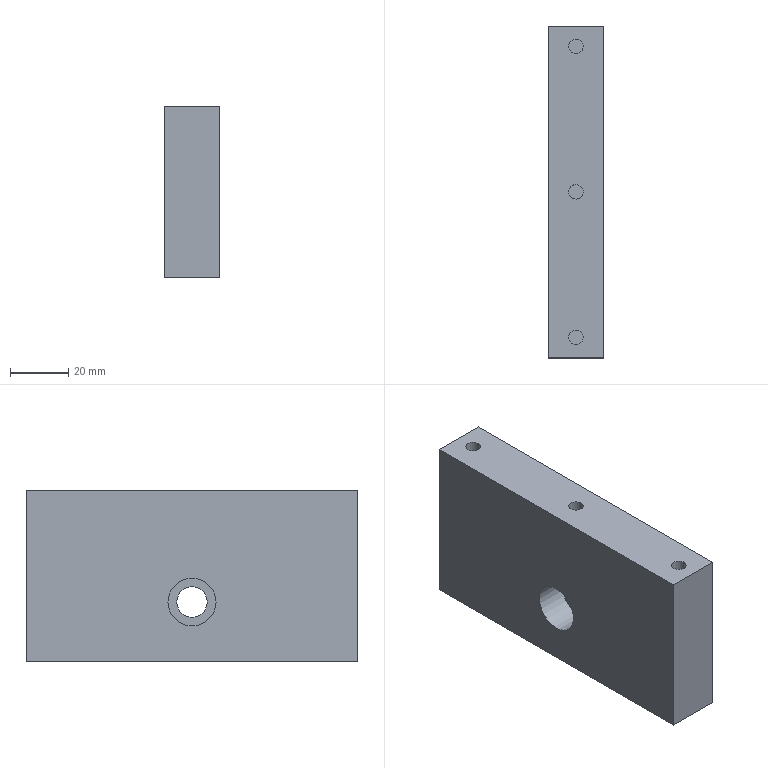CAM job | NX | 3+2 milling, drilling | part box 19 x 114 x 59 mm | stock box 25 x 119 x 60 mm
Tools:
number,name,description,diameter,corner_radius,flute_length,length,flutes
6,D6,平底铣刀-粗,6.0,0.0,25.0,75.0,2
9,D10,平底铣刀-粗,10.0,0.0,35.0,75.0,2
7,D6-J,平底铣刀-精,6.0,0.0,25.0,75.0,2
10,D10-J,平底铣刀-精,10.0,0.0,35.0,75.0,2
1,D80R0.8飞刀,圆鼻刀-粗,80.0,0.8,50.0,75.0,2
1,D80R0.8飞刀-J,圆鼻刀-精,80.0,0.8,50.0,75.0,2
2,D6倒角刀,倒角刀,6.0,0.0,3.0,25.0,2
17,ZT10.5,钻头,10.5,0.0,35.0,50.0,2
Operations:
program,operation,operation_type,tool,method,geometry_group,spindle_rpm,surface_speed,feed_per_tooth,feed_cut,feed_plunge,cut_length_mm,path_length_mm,cut_time_min,machine_time_min
B,底壁铣飞面一刀开粗_COPY,VolumeBased25DMillingOperation,D80R0.8飞刀,分层开粗-切深K-步距G,W-B,2800.0,703.696,0.5357,3000.0,100.0,2444.134,4883.512,0.8147,1.059
B,底壁铣飞面一刀精光_COPY,VolumeBased25DMillingOperation,D80R0.8飞刀-J,侧刃精光-切深K-步距G,W-B,4000.0,1005.28,0.125,1000.0,100.0,221.998,257.998,0.222,0.2256
B,底壁铣分层开粗-中_COPY,VolumeBased25DMillingOperation,D6,分层开粗-切深K-步距G,W-B,8000.0,150.796,0.125,2000.0,100.0,542.306,594.381,0.2712,0.2764
B,平面去毛刺6X45L_COPY,SurfaceContour,D6倒角刀,爬面_倒角-切深0-步距G,W-B,6500.0,122.519,0.1154,1500.0,100.0,386.393,475.439,0.2576,0.2665
B,底壁铣倒角_COPY,VolumeBased25DMillingOperation,D6倒角刀,爬面_倒角-切深0-步距G,W-B,6500.0,122.519,0.1154,1500.0,100.0,83.049,121.849,0.0554,0.0592
B,底壁铣精光底面-中_COPY,VolumeBased25DMillingOperation,D6-J,精光步距切深关,W-B,8000.0,150.792,0.0625,1000.0,100.0,114.555,146.655,0.1146,0.1178
B,底壁铣精光侧面-中-选底面_COPY,VolumeBased25DMillingOperation,D6-J,侧刃精光-切深K-步距G,W-B,8000.0,150.792,0.0625,1000.0,100.0,68.165,101.765,0.0682,0.0715
A,顶面,FaceMilling,D80R0.8飞刀,侧刃精光-切深K-步距G,W-A,5000.0,1256.637,0.1,1000.0,100.0,208.0,244.0,0.208,0.2116
A,外形粗_2,VolumeBased25DMillingOperation,D10,METHOD,W-A,8000.0,251.327,0.3125,5000.0,80.0,9830.672,9888.672,1.966,1.972
A,沉头孔打点-深0.8,Operation,D6倒角刀,NONE,W-A,8000.0,150.796,0.0312,500.0,90.0,1.8,43.6,0.0036,0.0078
A,沉头孔-钻孔0段,Operation,ZT10.5,NONE,W-A,1500.0,49.48,0.0833,250.0,90.0,24.0,88.0,0.096,0.1024
A,铣孔开粗D8_1,CylinderMilling,D10,NONE,W-A,8000.0,201.062,0.075,1200.0,100.0,485.05,535.55,0.4042,0.4093
A,仅选体,SurfaceContour,D6倒角刀,METHOD,W-A,8000.0,150.796,0.1875,3000.0,100.0,416.188,504.269,0.1387,0.1475
A,铣倒角_1,PlanarMilling,D6倒角刀,NONE,W-A,8000.0,150.796,0.05,800.0,100.0,60.671,96.671,0.0758,0.0794
A,铣孔精光D8_1,CylinderMilling,D10-J,精光步距切深关,W-A,8000.0,201.062,0.0312,500.0,100.0,78.948,129.448,0.1579,0.1629
A,外形半精_2,VolumeBased25DMillingOperation,D10-J,METHOD,W-A,8000.0,251.327,0.0625,1000.0,100.0,382.374,460.374,0.3824,0.3902